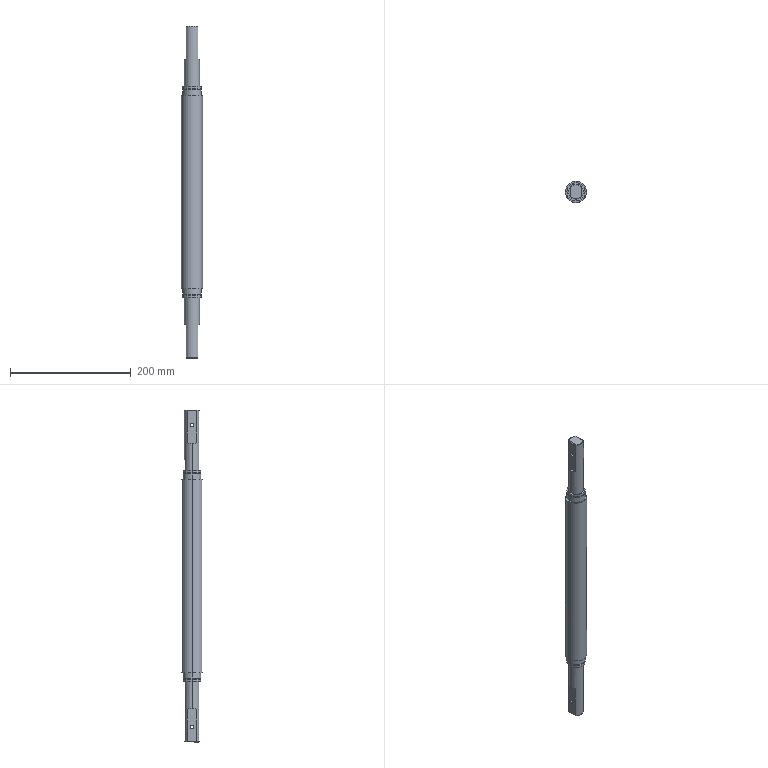Part | STEP file | Shaft 2 | 1 solid | 49 faces | box 35 x 35 x 550 mm | volume 418334 mm3 | cylinder 22 | plane 22 | cone 5 | commonest cylinder face diameters 30 x8 6 x4 25 x4 27.6 x4 35 x2
STEP:
#1=CARTESIAN_POINT('',(-17.5,0.,335.));
#2=VERTEX_POINT('',#1);
#3=CARTESIAN_POINT('',(17.5,0.,335.));
#4=VERTEX_POINT('',#3);
#5=CARTESIAN_POINT('',(0.,0.,335.));
#6=DIRECTION('',(0.,0.,-1.));
#7=DIRECTION('',(-1.,0.,0.));
#8=AXIS2_PLACEMENT_3D('',#5,#6,#7);
#9=CIRCLE('',#8,17.5);
#10=EDGE_CURVE('',#2,#4,#9,.T.);
#11=ORIENTED_EDGE('',*,*,#10,.T.);
#12=CARTESIAN_POINT('',(17.5,0.,15.));
#13=VERTEX_POINT('',#12);
#14=CARTESIAN_POINT('',(17.5,0.,350.));
#15=DIRECTION('',(0.,0.,-1.));
#16=VECTOR('',#15,1000.);
#17=LINE('',#14,#16);
#18=EDGE_CURVE('',#4,#13,#17,.T.);
#19=ORIENTED_EDGE('',*,*,#18,.T.);
#20=CARTESIAN_POINT('',(-17.5,0.,15.));
#21=VERTEX_POINT('',#20);
#22=CARTESIAN_POINT('',(0.,0.,15.));
#23=DIRECTION('',(0.,0.,1.));
#24=DIRECTION('',(-1.,0.,0.));
#25=AXIS2_PLACEMENT_3D('',#22,#23,#24);
#26=CIRCLE('',#25,17.5);
#27=EDGE_CURVE('',#13,#21,#26,.T.);
#28=ORIENTED_EDGE('',*,*,#27,.T.);
#29=CARTESIAN_POINT('',(-17.5,0.,350.));
#30=DIRECTION('',(0.,0.,-1.));
#31=VECTOR('',#30,1000.);
#32=LINE('',#29,#31);
#33=EDGE_CURVE('',#2,#21,#32,.T.);
#34=ORIENTED_EDGE('',*,*,#33,.F.);
#35=EDGE_LOOP('',(#11,#19,#28,#34));
#36=FACE_OUTER_BOUND('',#35,.T.);
#37=CARTESIAN_POINT('',(0.,0.,350.));
#38=DIRECTION('',(0.,0.,-1.));
#39=DIRECTION('',(-1.,0.,0.));
#40=AXIS2_PLACEMENT_3D('',#37,#38,#39);
#41=CYLINDRICAL_SURFACE('',#40,17.5);
#42=ADVANCED_FACE('',(#36),#41,.T.);
#43=CARTESIAN_POINT('',(15.,0.,15.));
#44=VERTEX_POINT('',#43);
#45=CARTESIAN_POINT('',(-15.,0.,15.));
#46=VERTEX_POINT('',#45);
#47=CARTESIAN_POINT('',(0.,0.,15.));
#48=DIRECTION('',(0.,0.,1.));
#49=DIRECTION('',(-1.,0.,0.));
#50=AXIS2_PLACEMENT_3D('',#47,#48,#49);
#51=CIRCLE('',#50,15.);
#52=EDGE_CURVE('',#44,#46,#51,.T.);
#53=ORIENTED_EDGE('',*,*,#52,.F.);
#54=CARTESIAN_POINT('',(15.,0.,6.));
#55=VERTEX_POINT('',#54);
#56=CARTESIAN_POINT('',(15.,0.,15.));
#57=DIRECTION('',(0.,0.,-1.));
#58=VECTOR('',#57,1000.);
#59=LINE('',#56,#58);
#60=EDGE_CURVE('',#44,#55,#59,.T.);
#61=ORIENTED_EDGE('',*,*,#60,.T.);
#62=CARTESIAN_POINT('',(-15.,0.,6.));
#63=VERTEX_POINT('',#62);
#64=CARTESIAN_POINT('',(0.,0.,6.));
#65=DIRECTION('',(0.,0.,1.));
#66=DIRECTION('',(-1.,0.,0.));
#67=AXIS2_PLACEMENT_3D('',#64,#65,#66);
#68=CIRCLE('',#67,15.);
#69=EDGE_CURVE('',#55,#63,#68,.T.);
#70=ORIENTED_EDGE('',*,*,#69,.T.);
#71=CARTESIAN_POINT('',(-15.,0.,15.));
#72=DIRECTION('',(0.,0.,-1.));
#73=VECTOR('',#72,1000.);
#74=LINE('',#71,#73);
#75=EDGE_CURVE('',#46,#63,#74,.T.);
#76=ORIENTED_EDGE('',*,*,#75,.F.);
#77=EDGE_LOOP('',(#53,#61,#70,#76));
#78=FACE_OUTER_BOUND('',#77,.T.);
#79=CARTESIAN_POINT('',(0.,0.,15.));
#80=DIRECTION('',(0.,0.,-1.));
#81=DIRECTION('',(-1.,0.,0.));
#82=AXIS2_PLACEMENT_3D('',#79,#80,#81);
#83=CYLINDRICAL_SURFACE('',#82,15.);
#84=ADVANCED_FACE('',(#78),#83,.T.);
#85=CARTESIAN_POINT('',(-15.,0.,335.));
#86=VERTEX_POINT('',#85);
#87=CARTESIAN_POINT('',(15.,0.,335.));
#88=VERTEX_POINT('',#87);
#89=CARTESIAN_POINT('',(0.,0.,335.));
#90=DIRECTION('',(0.,0.,-1.));
#91=DIRECTION('',(1.,0.,0.));
#92=AXIS2_PLACEMENT_3D('',#89,#90,#91);
#93=CIRCLE('',#92,15.);
#94=EDGE_CURVE('',#86,#88,#93,.T.);
#95=ORIENTED_EDGE('',*,*,#94,.F.);
#96=CARTESIAN_POINT('',(-15.,0.,344.));
#97=VERTEX_POINT('',#96);
#98=CARTESIAN_POINT('',(-15.,0.,335.));
#99=DIRECTION('',(0.,0.,1.));
#100=VECTOR('',#99,1000.);
#101=LINE('',#98,#100);
#102=EDGE_CURVE('',#86,#97,#101,.T.);
#103=ORIENTED_EDGE('',*,*,#102,.T.);
#104=CARTESIAN_POINT('',(15.,0.,344.));
#105=VERTEX_POINT('',#104);
#106=CARTESIAN_POINT('',(0.,0.,344.));
#107=DIRECTION('',(0.,0.,-1.));
#108=DIRECTION('',(1.,0.,0.));
#109=AXIS2_PLACEMENT_3D('',#106,#107,#108);
#110=CIRCLE('',#109,15.);
#111=EDGE_CURVE('',#97,#105,#110,.T.);
#112=ORIENTED_EDGE('',*,*,#111,.T.);
#113=CARTESIAN_POINT('',(15.,0.,335.));
#114=DIRECTION('',(0.,0.,1.));
#115=VECTOR('',#114,1000.);
#116=LINE('',#113,#115);
#117=EDGE_CURVE('',#88,#105,#116,.T.);
#118=ORIENTED_EDGE('',*,*,#117,.F.);
#119=EDGE_LOOP('',(#95,#103,#112,#118));
#120=FACE_OUTER_BOUND('',#119,.T.);
#121=CARTESIAN_POINT('',(0.,0.,335.));
#122=DIRECTION('',(0.,0.,1.));
#123=DIRECTION('',(1.,0.,0.));
#124=AXIS2_PLACEMENT_3D('',#121,#122,#123);
#125=CYLINDRICAL_SURFACE('',#124,15.);
#126=ADVANCED_FACE('',(#120),#125,.T.);
#127=CARTESIAN_POINT('',(-13.8,0.,6.));
#128=VERTEX_POINT('',#127);
#129=CARTESIAN_POINT('',(13.8,0.,6.));
#130=VERTEX_POINT('',#129);
#131=CARTESIAN_POINT('',(0.,0.,6.));
#132=DIRECTION('',(0.,0.,-1.));
#133=DIRECTION('',(-1.,0.,0.));
#134=AXIS2_PLACEMENT_3D('',#131,#132,#133);
#135=CIRCLE('',#134,13.8);
#136=EDGE_CURVE('',#128,#130,#135,.T.);
#137=ORIENTED_EDGE('',*,*,#136,.T.);
#138=CARTESIAN_POINT('',(13.8,0.,4.));
#139=VERTEX_POINT('',#138);
#140=CARTESIAN_POINT('',(13.8,0.,-86.604));
#141=DIRECTION('',(0.,0.,-1.));
#142=VECTOR('',#141,1000.);
#143=LINE('',#140,#142);
#144=EDGE_CURVE('',#130,#139,#143,.T.);
#145=ORIENTED_EDGE('',*,*,#144,.T.);
#146=CARTESIAN_POINT('',(-13.8,0.,4.));
#147=VERTEX_POINT('',#146);
#148=CARTESIAN_POINT('',(0.,0.,4.));
#149=DIRECTION('',(0.,0.,1.));
#150=DIRECTION('',(-1.,0.,0.));
#151=AXIS2_PLACEMENT_3D('',#148,#149,#150);
#152=CIRCLE('',#151,13.8);
#153=EDGE_CURVE('',#139,#147,#152,.T.);
#154=ORIENTED_EDGE('',*,*,#153,.T.);
#155=CARTESIAN_POINT('',(-13.8,0.,-86.604));
#156=DIRECTION('',(0.,0.,-1.));
#157=VECTOR('',#156,1000.);
#158=LINE('',#155,#157);
#159=EDGE_CURVE('',#128,#147,#158,.T.);
#160=ORIENTED_EDGE('',*,*,#159,.F.);
#161=EDGE_LOOP('',(#137,#145,#154,#160));
#162=FACE_OUTER_BOUND('',#161,.T.);
#163=CARTESIAN_POINT('',(0.,0.,-86.604));
#164=DIRECTION('',(0.,0.,-1.));
#165=DIRECTION('',(-1.,0.,0.));
#166=AXIS2_PLACEMENT_3D('',#163,#164,#165);
#167=CYLINDRICAL_SURFACE('',#166,13.8);
#168=ADVANCED_FACE('',(#162),#167,.T.);
#169=CARTESIAN_POINT('',(-13.8,0.,346.));
#170=VERTEX_POINT('',#169);
#171=CARTESIAN_POINT('',(13.8,0.,346.));
#172=VERTEX_POINT('',#171);
#173=CARTESIAN_POINT('',(0.,0.,346.));
#174=DIRECTION('',(0.,0.,-1.));
#175=DIRECTION('',(-1.,0.,0.));
#176=AXIS2_PLACEMENT_3D('',#173,#174,#175);
#177=CIRCLE('',#176,13.8);
#178=EDGE_CURVE('',#170,#172,#177,.T.);
#179=ORIENTED_EDGE('',*,*,#178,.T.);
#180=CARTESIAN_POINT('',(13.8,0.,344.));
#181=VERTEX_POINT('',#180);
#182=CARTESIAN_POINT('',(13.8,0.,-86.604));
#183=DIRECTION('',(0.,0.,-1.));
#184=VECTOR('',#183,1000.);
#185=LINE('',#182,#184);
#186=EDGE_CURVE('',#172,#181,#185,.T.);
#187=ORIENTED_EDGE('',*,*,#186,.T.);
#188=CARTESIAN_POINT('',(-13.8,0.,344.));
#189=VERTEX_POINT('',#188);
#190=CARTESIAN_POINT('',(0.,0.,344.));
#191=DIRECTION('',(0.,0.,1.));
#192=DIRECTION('',(-1.,0.,0.));
#193=AXIS2_PLACEMENT_3D('',#190,#191,#192);
#194=CIRCLE('',#193,13.8);
#195=EDGE_CURVE('',#181,#189,#194,.T.);
#196=ORIENTED_EDGE('',*,*,#195,.T.);
#197=CARTESIAN_POINT('',(-13.8,0.,-86.604));
#198=DIRECTION('',(0.,0.,-1.));
#199=VECTOR('',#198,1000.);
#200=LINE('',#197,#199);
#201=EDGE_CURVE('',#170,#189,#200,.T.);
#202=ORIENTED_EDGE('',*,*,#201,.F.);
#203=EDGE_LOOP('',(#179,#187,#196,#202));
#204=FACE_OUTER_BOUND('',#203,.T.);
#205=CARTESIAN_POINT('',(0.,0.,-86.604));
#206=DIRECTION('',(0.,0.,-1.));
#207=DIRECTION('',(-1.,0.,0.));
#208=AXIS2_PLACEMENT_3D('',#205,#206,#207);
#209=CYLINDRICAL_SURFACE('',#208,13.8);
#210=ADVANCED_FACE('',(#204),#209,.T.);
#211=CARTESIAN_POINT('',(-15.,0.,4.));
#212=VERTEX_POINT('',#211);
#213=CARTESIAN_POINT('',(15.,0.,4.));
#214=VERTEX_POINT('',#213);
#215=CARTESIAN_POINT('',(0.,0.,4.));
#216=DIRECTION('',(0.,0.,-1.));
#217=DIRECTION('',(-1.,0.,0.));
#218=AXIS2_PLACEMENT_3D('',#215,#216,#217);
#219=CIRCLE('',#218,15.);
#220=EDGE_CURVE('',#212,#214,#219,.T.);
#221=ORIENTED_EDGE('',*,*,#220,.T.);
#222=CARTESIAN_POINT('',(15.,0.,0.));
#223=VERTEX_POINT('',#222);
#224=CARTESIAN_POINT('',(15.,0.,15.));
#225=DIRECTION('',(0.,0.,-1.));
#226=VECTOR('',#225,1000.);
#227=LINE('',#224,#226);
#228=EDGE_CURVE('',#214,#223,#227,.T.);
#229=ORIENTED_EDGE('',*,*,#228,.T.);
#230=CARTESIAN_POINT('',(-15.,0.,0.));
#231=VERTEX_POINT('',#230);
#232=CARTESIAN_POINT('',(0.,0.,0.));
#233=DIRECTION('',(0.,0.,1.));
#234=DIRECTION('',(-1.,0.,0.));
#235=AXIS2_PLACEMENT_3D('',#232,#233,#234);
#236=CIRCLE('',#235,15.);
#237=EDGE_CURVE('',#223,#231,#236,.T.);
#238=ORIENTED_EDGE('',*,*,#237,.T.);
#239=CARTESIAN_POINT('',(-15.,0.,15.));
#240=DIRECTION('',(0.,0.,-1.));
#241=VECTOR('',#240,1000.);
#242=LINE('',#239,#241);
#243=EDGE_CURVE('',#212,#231,#242,.T.);
#244=ORIENTED_EDGE('',*,*,#243,.F.);
#245=EDGE_LOOP('',(#221,#229,#238,#244));
#246=FACE_OUTER_BOUND('',#245,.T.);
#247=CARTESIAN_POINT('',(0.,0.,15.));
#248=DIRECTION('',(0.,0.,-1.));
#249=DIRECTION('',(-1.,0.,0.));
#250=AXIS2_PLACEMENT_3D('',#247,#248,#249);
#251=CYLINDRICAL_SURFACE('',#250,15.);
#252=ADVANCED_FACE('',(#246),#251,.T.);
#253=CARTESIAN_POINT('',(15.,0.,346.));
#254=VERTEX_POINT('',#253);
#255=CARTESIAN_POINT('',(-15.,0.,346.));
#256=VERTEX_POINT('',#255);
#257=CARTESIAN_POINT('',(0.,0.,346.));
#258=DIRECTION('',(0.,0.,1.));
#259=DIRECTION('',(1.,0.,0.));
#260=AXIS2_PLACEMENT_3D('',#257,#258,#259);
#261=CIRCLE('',#260,15.);
#262=EDGE_CURVE('',#254,#256,#261,.T.);
#263=ORIENTED_EDGE('',*,*,#262,.T.);
#264=CARTESIAN_POINT('',(-15.,0.,350.));
#265=VERTEX_POINT('',#264);
#266=CARTESIAN_POINT('',(-15.,0.,335.));
#267=DIRECTION('',(0.,0.,1.));
#268=VECTOR('',#267,1000.);
#269=LINE('',#266,#268);
#270=EDGE_CURVE('',#256,#265,#269,.T.);
#271=ORIENTED_EDGE('',*,*,#270,.T.);
#272=CARTESIAN_POINT('',(15.,0.,350.));
#273=VERTEX_POINT('',#272);
#274=CARTESIAN_POINT('',(0.,0.,350.));
#275=DIRECTION('',(0.,0.,-1.));
#276=DIRECTION('',(1.,0.,0.));
#277=AXIS2_PLACEMENT_3D('',#274,#275,#276);
#278=CIRCLE('',#277,15.);
#279=EDGE_CURVE('',#265,#273,#278,.T.);
#280=ORIENTED_EDGE('',*,*,#279,.T.);
#281=CARTESIAN_POINT('',(15.,0.,335.));
#282=DIRECTION('',(0.,0.,1.));
#283=VECTOR('',#282,1000.);
#284=LINE('',#281,#283);
#285=EDGE_CURVE('',#254,#273,#284,.T.);
#286=ORIENTED_EDGE('',*,*,#285,.F.);
#287=EDGE_LOOP('',(#263,#271,#280,#286));
#288=FACE_OUTER_BOUND('',#287,.T.);
#289=CARTESIAN_POINT('',(0.,0.,335.));
#290=DIRECTION('',(0.,0.,1.));
#291=DIRECTION('',(1.,0.,0.));
#292=AXIS2_PLACEMENT_3D('',#289,#290,#291);
#293=CYLINDRICAL_SURFACE('',#292,15.);
#294=ADVANCED_FACE('',(#288),#293,.T.);
#295=CARTESIAN_POINT('',(-9.5,8.124,-45.));
#296=VERTEX_POINT('',#295);
#297=CARTESIAN_POINT('',(-12.5,0.,-45.));
#298=VERTEX_POINT('',#297);
#299=CARTESIAN_POINT('',(0.,0.,-45.));
#300=DIRECTION('',(0.,0.,1.));
#301=DIRECTION('',(1.,0.,0.));
#302=AXIS2_PLACEMENT_3D('',#299,#300,#301);
#303=CIRCLE('',#302,12.5);
#304=EDGE_CURVE('',#296,#298,#303,.T.);
#305=ORIENTED_EDGE('',*,*,#304,.T.);
#306=CARTESIAN_POINT('',(-12.5,0.,0.));
#307=VERTEX_POINT('',#306);
#308=CARTESIAN_POINT('',(-12.5,0.,-100.));
#309=DIRECTION('',(0.,0.,1.));
#310=VECTOR('',#309,1000.);
#311=LINE('',#308,#310);
#312=EDGE_CURVE('',#298,#307,#311,.T.);
#313=ORIENTED_EDGE('',*,*,#312,.T.);
#314=CARTESIAN_POINT('',(12.5,0.,0.));
#315=VERTEX_POINT('',#314);
#316=CARTESIAN_POINT('',(0.,0.,0.));
#317=DIRECTION('',(0.,0.,-1.));
#318=DIRECTION('',(1.,0.,0.));
#319=AXIS2_PLACEMENT_3D('',#316,#317,#318);
#320=CIRCLE('',#319,12.5);
#321=EDGE_CURVE('',#307,#315,#320,.T.);
#322=ORIENTED_EDGE('',*,*,#321,.T.);
#323=CARTESIAN_POINT('',(12.5,0.,-45.));
#324=VERTEX_POINT('',#323);
#325=CARTESIAN_POINT('',(12.5,0.,-100.));
#326=DIRECTION('',(0.,0.,1.));
#327=VECTOR('',#326,1000.);
#328=LINE('',#325,#327);
#329=EDGE_CURVE('',#324,#315,#328,.T.);
#330=ORIENTED_EDGE('',*,*,#329,.F.);
#331=CARTESIAN_POINT('',(9.5,8.124,-45.));
#332=VERTEX_POINT('',#331);
#333=CARTESIAN_POINT('',(0.,0.,-45.));
#334=DIRECTION('',(0.,0.,1.));
#335=DIRECTION('',(1.,0.,0.));
#336=AXIS2_PLACEMENT_3D('',#333,#334,#335);
#337=CIRCLE('',#336,12.5);
#338=EDGE_CURVE('',#324,#332,#337,.T.);
#339=ORIENTED_EDGE('',*,*,#338,.T.);
#340=CARTESIAN_POINT('',(9.5,8.124,-99.));
#341=VERTEX_POINT('',#340);
#342=CARTESIAN_POINT('',(9.5,8.124,-100.));
#343=DIRECTION('',(0.,0.,-1.));
#344=VECTOR('',#343,1000.);
#345=LINE('',#342,#344);
#346=EDGE_CURVE('',#332,#341,#345,.T.);
#347=ORIENTED_EDGE('',*,*,#346,.T.);
#348=CARTESIAN_POINT('',(-9.5,8.124,-99.));
#349=VERTEX_POINT('',#348);
#350=CARTESIAN_POINT('',(0.,0.,-99.));
#351=DIRECTION('',(0.,0.,1.));
#352=DIRECTION('',(1.,0.,0.));
#353=AXIS2_PLACEMENT_3D('',#350,#351,#352);
#354=CIRCLE('',#353,12.5);
#355=EDGE_CURVE('',#341,#349,#354,.T.);
#356=ORIENTED_EDGE('',*,*,#355,.T.);
#357=CARTESIAN_POINT('',(-9.5,8.124,-100.));
#358=DIRECTION('',(0.,0.,1.));
#359=VECTOR('',#358,1000.);
#360=LINE('',#357,#359);
#361=EDGE_CURVE('',#349,#296,#360,.T.);
#362=ORIENTED_EDGE('',*,*,#361,.T.);
#363=EDGE_LOOP('',(#305,#313,#322,#330,#339,#347,#356,#362));
#364=FACE_OUTER_BOUND('',#363,.T.);
#365=CARTESIAN_POINT('',(0.,0.,-100.));
#366=DIRECTION('',(0.,0.,1.));
#367=DIRECTION('',(1.,0.,0.));
#368=AXIS2_PLACEMENT_3D('',#365,#366,#367);
#369=CYLINDRICAL_SURFACE('',#368,12.5);
#370=ADVANCED_FACE('',(#364),#369,.T.);
#371=CARTESIAN_POINT('',(9.5,8.124,395.));
#372=VERTEX_POINT('',#371);
#373=CARTESIAN_POINT('',(12.5,0.,395.));
#374=VERTEX_POINT('',#373);
#375=CARTESIAN_POINT('',(0.,0.,395.));
#376=DIRECTION('',(0.,0.,-1.));
#377=DIRECTION('',(-1.,0.,0.));
#378=AXIS2_PLACEMENT_3D('',#375,#376,#377);
#379=CIRCLE('',#378,12.5);
#380=EDGE_CURVE('',#372,#374,#379,.T.);
#381=ORIENTED_EDGE('',*,*,#380,.T.);
#382=CARTESIAN_POINT('',(12.5,0.,350.));
#383=VERTEX_POINT('',#382);
#384=CARTESIAN_POINT('',(12.5,0.,450.));
#385=DIRECTION('',(0.,0.,-1.));
#386=VECTOR('',#385,1000.);
#387=LINE('',#384,#386);
#388=EDGE_CURVE('',#374,#383,#387,.T.);
#389=ORIENTED_EDGE('',*,*,#388,.T.);
#390=CARTESIAN_POINT('',(-12.5,0.,350.));
#391=VERTEX_POINT('',#390);
#392=CARTESIAN_POINT('',(0.,0.,350.));
#393=DIRECTION('',(0.,0.,-1.));
#394=DIRECTION('',(-1.,0.,0.));
#395=AXIS2_PLACEMENT_3D('',#392,#393,#394);
#396=CIRCLE('',#395,12.5);
#397=EDGE_CURVE('',#391,#383,#396,.T.);
#398=ORIENTED_EDGE('',*,*,#397,.F.);
#399=CARTESIAN_POINT('',(-12.5,0.,395.));
#400=VERTEX_POINT('',#399);
#401=CARTESIAN_POINT('',(-12.5,0.,450.));
#402=DIRECTION('',(0.,0.,-1.));
#403=VECTOR('',#402,1000.);
#404=LINE('',#401,#403);
#405=EDGE_CURVE('',#400,#391,#404,.T.);
#406=ORIENTED_EDGE('',*,*,#405,.F.);
#407=CARTESIAN_POINT('',(-9.5,8.124,395.));
#408=VERTEX_POINT('',#407);
#409=CARTESIAN_POINT('',(0.,0.,395.));
#410=DIRECTION('',(0.,0.,-1.));
#411=DIRECTION('',(-1.,0.,0.));
#412=AXIS2_PLACEMENT_3D('',#409,#410,#411);
#413=CIRCLE('',#412,12.5);
#414=EDGE_CURVE('',#400,#408,#413,.T.);
#415=ORIENTED_EDGE('',*,*,#414,.T.);
#416=CARTESIAN_POINT('',(-9.5,8.124,449.));
#417=VERTEX_POINT('',#416);
#418=CARTESIAN_POINT('',(-9.5,8.124,450.));
#419=DIRECTION('',(0.,0.,1.));
#420=VECTOR('',#419,1000.);
#421=LINE('',#418,#420);
#422=EDGE_CURVE('',#408,#417,#421,.T.);
#423=ORIENTED_EDGE('',*,*,#422,.T.);
#424=CARTESIAN_POINT('',(0.,12.5,449.));
#425=VERTEX_POINT('',#424);
#426=CARTESIAN_POINT('',(0.,0.,449.));
#427=DIRECTION('',(0.,0.,-1.));
#428=DIRECTION('',(-1.,0.,0.));
#429=AXIS2_PLACEMENT_3D('',#426,#427,#428);
#430=CIRCLE('',#429,12.5);
#431=EDGE_CURVE('',#417,#425,#430,.T.);
#432=ORIENTED_EDGE('',*,*,#431,.T.);
#433=CARTESIAN_POINT('',(9.5,8.124,449.));
#434=VERTEX_POINT('',#433);
#435=CARTESIAN_POINT('',(0.,0.,449.));
#436=DIRECTION('',(0.,0.,-1.));
#437=DIRECTION('',(-1.,0.,0.));
#438=AXIS2_PLACEMENT_3D('',#435,#436,#437);
#439=CIRCLE('',#438,12.5);
#440=EDGE_CURVE('',#425,#434,#439,.T.);
#441=ORIENTED_EDGE('',*,*,#440,.T.);
#442=CARTESIAN_POINT('',(9.5,8.124,450.));
#443=DIRECTION('',(0.,0.,-1.));
#444=VECTOR('',#443,1000.);
#445=LINE('',#442,#444);
#446=EDGE_CURVE('',#434,#372,#445,.T.);
#447=ORIENTED_EDGE('',*,*,#446,.T.);
#448=EDGE_LOOP('',(#381,#389,#398,#406,#415,#423,#432,#441,#447));
#449=FACE_OUTER_BOUND('',#448,.T.);
#450=CARTESIAN_POINT('',(0.,0.,450.));
#451=DIRECTION('',(0.,0.,-1.));
#452=DIRECTION('',(-1.,0.,0.));
#453=AXIS2_PLACEMENT_3D('',#450,#451,#452);
#454=CYLINDRICAL_SURFACE('',#453,12.5);
#455=ADVANCED_FACE('',(#449),#454,.T.);
#456=CARTESIAN_POINT('',(-8.5,7.746,450.));
#457=VERTEX_POINT('',#456);
#458=CARTESIAN_POINT('',(0.,11.5,450.));
#459=VERTEX_POINT('',#458);
#460=CARTESIAN_POINT('',(0.,0.,450.));
#461=DIRECTION('',(0.,0.,-1.));
#462=DIRECTION('',(0.,1.,0.));
#463=AXIS2_PLACEMENT_3D('',#460,#461,#462);
#464=CIRCLE('',#463,11.5);
#465=EDGE_CURVE('',#457,#459,#464,.T.);
#466=ORIENTED_EDGE('',*,*,#465,.T.);
#467=CARTESIAN_POINT('',(0.,12.5,449.));
#468=DIRECTION('',(0.,0.7071,-0.7071));
#469=VECTOR('',#468,1000.);
#470=LINE('',#467,#469);
#471=EDGE_CURVE('',#459,#425,#470,.T.);
#472=ORIENTED_EDGE('',*,*,#471,.T.);
#473=ORIENTED_EDGE('',*,*,#431,.F.);
#474=CARTESIAN_POINT('',(-8.5,7.746,450.));
#475=CARTESIAN_POINT('',(-8.833,7.875,449.667));
#476=CARTESIAN_POINT('',(-9.166,8.001,449.334));
#477=CARTESIAN_POINT('',(-9.5,8.124,449.));
#478=B_SPLINE_CURVE_WITH_KNOTS('',3,(#474,#475,#476,#477),.UNSPECIFIED.,.F.,.F.,(4,4),(0.,0.001464),.UNSPECIFIED.);
#479=EDGE_CURVE('',#457,#417,#478,.T.);
#480=ORIENTED_EDGE('',*,*,#479,.F.);
#481=EDGE_LOOP('',(#466,#472,#473,#480));
#482=FACE_OUTER_BOUND('',#481,.T.);
#483=CARTESIAN_POINT('',(0.,0.,449.));
#484=DIRECTION('',(0.,0.,-1.));
#485=DIRECTION('',(0.,1.,0.));
#486=AXIS2_PLACEMENT_3D('',#483,#484,#485);
#487=CONICAL_SURFACE('',#486,12.5,0.7854);
#488=ADVANCED_FACE('',(#482),#487,.T.);
#489=CARTESIAN_POINT('',(-9.5,0.,-78.));
#490=VERTEX_POINT('',#489);
#491=CARTESIAN_POINT('',(-9.5,0.,-72.));
#492=VERTEX_POINT('',#491);
#493=CARTESIAN_POINT('',(-9.5,0.,-75.));
#494=DIRECTION('',(-1.,0.,0.));
#495=DIRECTION('',(0.,0.,-1.));
#496=AXIS2_PLACEMENT_3D('',#493,#494,#495);
#497=CIRCLE('',#496,3.);
#498=EDGE_CURVE('',#490,#492,#497,.T.);
#499=ORIENTED_EDGE('',*,*,#498,.T.);
#500=CARTESIAN_POINT('',(9.5,0.,-72.));
#501=VERTEX_POINT('',#500);
#502=CARTESIAN_POINT('',(-10.5,0.,-72.));
#503=DIRECTION('',(1.,0.,0.));
#504=VECTOR('',#503,1000.);
#505=LINE('',#502,#504);
#506=EDGE_CURVE('',#492,#501,#505,.T.);
#507=ORIENTED_EDGE('',*,*,#506,.T.);
#508=CARTESIAN_POINT('',(9.5,0.,-78.));
#509=VERTEX_POINT('',#508);
#510=CARTESIAN_POINT('',(9.5,0.,-75.));
#511=DIRECTION('',(1.,0.,0.));
#512=DIRECTION('',(0.,0.,-1.));
#513=AXIS2_PLACEMENT_3D('',#510,#511,#512);
#514=CIRCLE('',#513,3.);
#515=EDGE_CURVE('',#501,#509,#514,.T.);
#516=ORIENTED_EDGE('',*,*,#515,.T.);
#517=CARTESIAN_POINT('',(-10.5,0.,-78.));
#518=DIRECTION('',(1.,0.,0.));
#519=VECTOR('',#518,1000.);
#520=LINE('',#517,#519);
#521=EDGE_CURVE('',#490,#509,#520,.T.);
#522=ORIENTED_EDGE('',*,*,#521,.F.);
#523=EDGE_LOOP('',(#499,#507,#516,#522));
#524=FACE_OUTER_BOUND('',#523,.T.);
#525=CARTESIAN_POINT('',(-10.5,0.,-75.));
#526=DIRECTION('',(1.,0.,0.));
#527=DIRECTION('',(0.,0.,-1.));
#528=AXIS2_PLACEMENT_3D('',#525,#526,#527);
#529=CYLINDRICAL_SURFACE('',#528,3.);
#530=ADVANCED_FACE('',(#524),#529,.F.);
#531=CARTESIAN_POINT('',(-9.5,0.,422.));
#532=VERTEX_POINT('',#531);
#533=CARTESIAN_POINT('',(-9.5,0.,428.));
#534=VERTEX_POINT('',#533);
#535=CARTESIAN_POINT('',(-9.5,0.,425.));
#536=DIRECTION('',(-1.,0.,0.));
#537=DIRECTION('',(0.,0.,-1.));
#538=AXIS2_PLACEMENT_3D('',#535,#536,#537);
#539=CIRCLE('',#538,3.);
#540=EDGE_CURVE('',#532,#534,#539,.T.);
#541=ORIENTED_EDGE('',*,*,#540,.T.);
#542=CARTESIAN_POINT('',(9.5,0.,428.));
#543=VERTEX_POINT('',#542);
#544=CARTESIAN_POINT('',(-10.5,0.,428.));
#545=DIRECTION('',(1.,0.,0.));
#546=VECTOR('',#545,1000.);
#547=LINE('',#544,#546);
#548=EDGE_CURVE('',#534,#543,#547,.T.);
#549=ORIENTED_EDGE('',*,*,#548,.T.);
#550=CARTESIAN_POINT('',(9.5,0.,422.));
#551=VERTEX_POINT('',#550);
#552=CARTESIAN_POINT('',(9.5,0.,425.));
#553=DIRECTION('',(1.,0.,0.));
#554=DIRECTION('',(0.,0.,-1.));
#555=AXIS2_PLACEMENT_3D('',#552,#553,#554);
#556=CIRCLE('',#555,3.);
#557=EDGE_CURVE('',#543,#551,#556,.T.);
#558=ORIENTED_EDGE('',*,*,#557,.T.);
#559=CARTESIAN_POINT('',(-10.5,0.,422.));
#560=DIRECTION('',(1.,0.,0.));
#561=VECTOR('',#560,1000.);
#562=LINE('',#559,#561);
#563=EDGE_CURVE('',#532,#551,#562,.T.);
#564=ORIENTED_EDGE('',*,*,#563,.F.);
#565=EDGE_LOOP('',(#541,#549,#558,#564));
#566=FACE_OUTER_BOUND('',#565,.T.);
#567=CARTESIAN_POINT('',(-10.5,0.,425.));
#568=DIRECTION('',(1.,0.,0.));
#569=DIRECTION('',(0.,0.,-1.));
#570=AXIS2_PLACEMENT_3D('',#567,#568,#569);
#571=CYLINDRICAL_SURFACE('',#570,3.);
#572=ADVANCED_FACE('',(#566),#571,.F.);
#573=ORIENTED_EDGE('',*,*,#18,.F.);
#574=CARTESIAN_POINT('',(0.,0.,335.));
#575=DIRECTION('',(0.,0.,-1.));
#576=DIRECTION('',(-1.,0.,0.));
#577=AXIS2_PLACEMENT_3D('',#574,#575,#576);
#578=CIRCLE('',#577,17.5);
#579=EDGE_CURVE('',#4,#2,#578,.T.);
#580=ORIENTED_EDGE('',*,*,#579,.T.);
#581=ORIENTED_EDGE('',*,*,#33,.T.);
#582=CARTESIAN_POINT('',(0.,0.,15.));
#583=DIRECTION('',(0.,0.,1.));
#584=DIRECTION('',(-1.,0.,0.));
#585=AXIS2_PLACEMENT_3D('',#582,#583,#584);
#586=CIRCLE('',#585,17.5);
#587=EDGE_CURVE('',#21,#13,#586,.T.);
#588=ORIENTED_EDGE('',*,*,#587,.T.);
#589=EDGE_LOOP('',(#573,#580,#581,#588));
#590=FACE_OUTER_BOUND('',#589,.T.);
#591=CARTESIAN_POINT('',(0.,0.,350.));
#592=DIRECTION('',(0.,0.,-1.));
#593=DIRECTION('',(-1.,0.,0.));
#594=AXIS2_PLACEMENT_3D('',#591,#592,#593);
#595=CYLINDRICAL_SURFACE('',#594,17.5);
#596=ADVANCED_FACE('',(#590),#595,.T.);
#597=ORIENTED_EDGE('',*,*,#587,.F.);
#598=ORIENTED_EDGE('',*,*,#27,.F.);
#599=EDGE_LOOP('',(#597,#598));
#600=FACE_OUTER_BOUND('',#599,.T.);
#601=CARTESIAN_POINT('',(0.,0.,15.));
#602=DIRECTION('',(0.,0.,1.));
#603=DIRECTION('',(-1.,0.,0.));
#604=AXIS2_PLACEMENT_3D('',#601,#602,#603);
#605=CIRCLE('',#604,15.);
#606=EDGE_CURVE('',#46,#44,#605,.T.);
#607=ORIENTED_EDGE('',*,*,#606,.T.);
#608=ORIENTED_EDGE('',*,*,#52,.T.);
#609=EDGE_LOOP('',(#607,#608));
#610=FACE_BOUND('',#609,.T.);
#611=CARTESIAN_POINT('',(0.,0.,15.));
#612=DIRECTION('',(0.,0.,-1.));
#613=DIRECTION('',(-1.,0.,0.));
#614=AXIS2_PLACEMENT_3D('',#611,#612,#613);
#615=PLANE('',#614);
#616=ADVANCED_FACE('',(#600,#610),#615,.T.);
#617=ORIENTED_EDGE('',*,*,#10,.F.);
#618=ORIENTED_EDGE('',*,*,#579,.F.);
#619=EDGE_LOOP('',(#617,#618));
#620=FACE_OUTER_BOUND('',#619,.T.);
#621=CARTESIAN_POINT('',(0.,0.,335.));
#622=DIRECTION('',(0.,0.,-1.));
#623=DIRECTION('',(1.,0.,0.));
#624=AXIS2_PLACEMENT_3D('',#621,#622,#623);
#625=CIRCLE('',#624,15.);
#626=EDGE_CURVE('',#88,#86,#625,.T.);
#627=ORIENTED_EDGE('',*,*,#626,.T.);
#628=ORIENTED_EDGE('',*,*,#94,.T.);
#629=EDGE_LOOP('',(#627,#628));
#630=FACE_BOUND('',#629,.T.);
#631=CARTESIAN_POINT('',(0.,0.,335.));
#632=DIRECTION('',(0.,0.,1.));
#633=DIRECTION('',(1.,0.,0.));
#634=AXIS2_PLACEMENT_3D('',#631,#632,#633);
#635=PLANE('',#634);
#636=ADVANCED_FACE('',(#620,#630),#635,.T.);
#637=ORIENTED_EDGE('',*,*,#60,.F.);
#638=ORIENTED_EDGE('',*,*,#606,.F.);
#639=ORIENTED_EDGE('',*,*,#75,.T.);
#640=CARTESIAN_POINT('',(0.,0.,6.));
#641=DIRECTION('',(0.,0.,1.));
#642=DIRECTION('',(-1.,0.,0.));
#643=AXIS2_PLACEMENT_3D('',#640,#641,#642);
#644=CIRCLE('',#643,15.);
#645=EDGE_CURVE('',#63,#55,#644,.T.);
#646=ORIENTED_EDGE('',*,*,#645,.T.);
#647=EDGE_LOOP('',(#637,#638,#639,#646));
#648=FACE_OUTER_BOUND('',#647,.T.);
#649=CARTESIAN_POINT('',(0.,0.,15.));
#650=DIRECTION('',(0.,0.,-1.));
#651=DIRECTION('',(-1.,0.,0.));
#652=AXIS2_PLACEMENT_3D('',#649,#650,#651);
#653=CYLINDRICAL_SURFACE('',#652,15.);
#654=ADVANCED_FACE('',(#648),#653,.T.);
#655=ORIENTED_EDGE('',*,*,#102,.F.);
#656=ORIENTED_EDGE('',*,*,#626,.F.);
#657=ORIENTED_EDGE('',*,*,#117,.T.);
#658=CARTESIAN_POINT('',(0.,0.,344.));
#659=DIRECTION('',(0.,0.,-1.));
#660=DIRECTION('',(1.,0.,0.));
#661=AXIS2_PLACEMENT_3D('',#658,#659,#660);
#662=CIRCLE('',#661,15.);
#663=EDGE_CURVE('',#105,#97,#662,.T.);
#664=ORIENTED_EDGE('',*,*,#663,.T.);
#665=EDGE_LOOP('',(#655,#656,#657,#664));
#666=FACE_OUTER_BOUND('',#665,.T.);
#667=CARTESIAN_POINT('',(0.,0.,335.));
#668=DIRECTION('',(0.,0.,1.));
#669=DIRECTION('',(1.,0.,0.));
#670=AXIS2_PLACEMENT_3D('',#667,#668,#669);
#671=CYLINDRICAL_SURFACE('',#670,15.);
#672=ADVANCED_FACE('',(#666),#671,.T.);
#673=ORIENTED_EDGE('',*,*,#136,.F.);
#674=CARTESIAN_POINT('',(0.,0.,6.));
#675=DIRECTION('',(0.,0.,-1.));
#676=DIRECTION('',(-1.,0.,0.));
#677=AXIS2_PLACEMENT_3D('',#674,#675,#676);
#678=CIRCLE('',#677,13.8);
#679=EDGE_CURVE('',#130,#128,#678,.T.);
#680=ORIENTED_EDGE('',*,*,#679,.F.);
#681=EDGE_LOOP('',(#673,#680));
#682=FACE_BOUND('',#681,.T.);
#683=ORIENTED_EDGE('',*,*,#645,.F.);
#684=ORIENTED_EDGE('',*,*,#69,.F.);
#685=EDGE_LOOP('',(#683,#684));
#686=FACE_OUTER_BOUND('',#685,.T.);
#687=CARTESIAN_POINT('',(-15.3,0.,6.));
#688=DIRECTION('',(0.,0.,1.));
#689=DIRECTION('',(1.,0.,0.));
#690=AXIS2_PLACEMENT_3D('',#687,#688,#689);
#691=PLANE('',#690);
#692=ADVANCED_FACE('',(#682,#686),#691,.F.);
#693=CARTESIAN_POINT('',(0.,0.,344.));
#694=DIRECTION('',(0.,0.,1.));
#695=DIRECTION('',(-1.,0.,0.));
#696=AXIS2_PLACEMENT_3D('',#693,#694,#695);
#697=CIRCLE('',#696,13.8);
#698=EDGE_CURVE('',#189,#181,#697,.T.);
#699=ORIENTED_EDGE('',*,*,#698,.F.);
#700=ORIENTED_EDGE('',*,*,#195,.F.);
#701=EDGE_LOOP('',(#699,#700));
#702=FACE_BOUND('',#701,.T.);
#703=ORIENTED_EDGE('',*,*,#663,.F.);
#704=ORIENTED_EDGE('',*,*,#111,.F.);
#705=EDGE_LOOP('',(#703,#704));
#706=FACE_OUTER_BOUND('',#705,.T.);
#707=CARTESIAN_POINT('',(-15.3,0.,344.));
#708=DIRECTION('',(0.,0.,-1.));
#709=DIRECTION('',(-1.,0.,0.));
#710=AXIS2_PLACEMENT_3D('',#707,#708,#709);
#711=PLANE('',#710);
#712=ADVANCED_FACE('',(#702,#706),#711,.F.);
#713=ORIENTED_EDGE('',*,*,#144,.F.);
#714=ORIENTED_EDGE('',*,*,#679,.T.);
#715=ORIENTED_EDGE('',*,*,#159,.T.);
#716=CARTESIAN_POINT('',(0.,0.,4.));
#717=DIRECTION('',(0.,0.,1.));
#718=DIRECTION('',(-1.,0.,0.));
#719=AXIS2_PLACEMENT_3D('',#716,#717,#718);
#720=CIRCLE('',#719,13.8);
#721=EDGE_CURVE('',#147,#139,#720,.T.);
#722=ORIENTED_EDGE('',*,*,#721,.T.);
#723=EDGE_LOOP('',(#713,#714,#715,#722));
#724=FACE_OUTER_BOUND('',#723,.T.);
#725=CARTESIAN_POINT('',(0.,0.,-86.604));
#726=DIRECTION('',(0.,0.,-1.));
#727=DIRECTION('',(-1.,0.,0.));
#728=AXIS2_PLACEMENT_3D('',#725,#726,#727);
#729=CYLINDRICAL_SURFACE('',#728,13.8);
#730=ADVANCED_FACE('',(#724),#729,.T.);
#731=ORIENTED_EDGE('',*,*,#186,.F.);
#732=CARTESIAN_POINT('',(0.,0.,346.));
#733=DIRECTION('',(0.,0.,-1.));
#734=DIRECTION('',(-1.,0.,0.));
#735=AXIS2_PLACEMENT_3D('',#732,#733,#734);
#736=CIRCLE('',#735,13.8);
#737=EDGE_CURVE('',#172,#170,#736,.T.);
#738=ORIENTED_EDGE('',*,*,#737,.T.);
#739=ORIENTED_EDGE('',*,*,#201,.T.);
#740=ORIENTED_EDGE('',*,*,#698,.T.);
#741=EDGE_LOOP('',(#731,#738,#739,#740));
#742=FACE_OUTER_BOUND('',#741,.T.);
#743=CARTESIAN_POINT('',(0.,0.,-86.604));
#744=DIRECTION('',(0.,0.,-1.));
#745=DIRECTION('',(-1.,0.,0.));
#746=AXIS2_PLACEMENT_3D('',#743,#744,#745);
#747=CYLINDRICAL_SURFACE('',#746,13.8);
#748=ADVANCED_FACE('',(#742),#747,.T.);
#749=ORIENTED_EDGE('',*,*,#721,.F.);
#750=ORIENTED_EDGE('',*,*,#153,.F.);
#751=EDGE_LOOP('',(#749,#750));
#752=FACE_BOUND('',#751,.T.);
#753=ORIENTED_EDGE('',*,*,#220,.F.);
#754=CARTESIAN_POINT('',(0.,0.,4.));
#755=DIRECTION('',(0.,0.,-1.));
#756=DIRECTION('',(-1.,0.,0.));
#757=AXIS2_PLACEMENT_3D('',#754,#755,#756);
#758=CIRCLE('',#757,15.);
#759=EDGE_CURVE('',#214,#212,#758,.T.);
#760=ORIENTED_EDGE('',*,*,#759,.F.);
#761=EDGE_LOOP('',(#753,#760));
#762=FACE_OUTER_BOUND('',#761,.T.);
#763=CARTESIAN_POINT('',(-15.3,0.,4.));
#764=DIRECTION('',(0.,0.,-1.));
#765=DIRECTION('',(-1.,0.,0.));
#766=AXIS2_PLACEMENT_3D('',#763,#764,#765);
#767=PLANE('',#766);
#768=ADVANCED_FACE('',(#752,#762),#767,.F.);
#769=ORIENTED_EDGE('',*,*,#178,.F.);
#770=ORIENTED_EDGE('',*,*,#737,.F.);
#771=EDGE_LOOP('',(#769,#770));
#772=FACE_BOUND('',#771,.T.);
#773=ORIENTED_EDGE('',*,*,#262,.F.);
#774=CARTESIAN_POINT('',(0.,0.,346.));
#775=DIRECTION('',(0.,0.,1.));
#776=DIRECTION('',(1.,0.,0.));
#777=AXIS2_PLACEMENT_3D('',#774,#775,#776);
#778=CIRCLE('',#777,15.);
#779=EDGE_CURVE('',#256,#254,#778,.T.);
#780=ORIENTED_EDGE('',*,*,#779,.F.);
#781=EDGE_LOOP('',(#773,#780));
#782=FACE_OUTER_BOUND('',#781,.T.);
#783=CARTESIAN_POINT('',(-15.3,0.,346.));
#784=DIRECTION('',(0.,0.,1.));
#785=DIRECTION('',(1.,0.,0.));
#786=AXIS2_PLACEMENT_3D('',#783,#784,#785);
#787=PLANE('',#786);
#788=ADVANCED_FACE('',(#772,#782),#787,.F.);
#789=ORIENTED_EDGE('',*,*,#228,.F.);
#790=ORIENTED_EDGE('',*,*,#759,.T.);
#791=ORIENTED_EDGE('',*,*,#243,.T.);
#792=CARTESIAN_POINT('',(0.,0.,0.));
#793=DIRECTION('',(0.,0.,1.));
#794=DIRECTION('',(-1.,0.,0.));
#795=AXIS2_PLACEMENT_3D('',#792,#793,#794);
#796=CIRCLE('',#795,15.);
#797=EDGE_CURVE('',#231,#223,#796,.T.);
#798=ORIENTED_EDGE('',*,*,#797,.T.);
#799=EDGE_LOOP('',(#789,#790,#791,#798));
#800=FACE_OUTER_BOUND('',#799,.T.);
#801=CARTESIAN_POINT('',(0.,0.,15.));
#802=DIRECTION('',(0.,0.,-1.));
#803=DIRECTION('',(-1.,0.,0.));
#804=AXIS2_PLACEMENT_3D('',#801,#802,#803);
#805=CYLINDRICAL_SURFACE('',#804,15.);
#806=ADVANCED_FACE('',(#800),#805,.T.);
#807=ORIENTED_EDGE('',*,*,#270,.F.);
#808=ORIENTED_EDGE('',*,*,#779,.T.);
#809=ORIENTED_EDGE('',*,*,#285,.T.);
#810=CARTESIAN_POINT('',(0.,0.,350.));
#811=DIRECTION('',(0.,0.,-1.));
#812=DIRECTION('',(1.,0.,0.));
#813=AXIS2_PLACEMENT_3D('',#810,#811,#812);
#814=CIRCLE('',#813,15.);
#815=EDGE_CURVE('',#273,#265,#814,.T.);
#816=ORIENTED_EDGE('',*,*,#815,.T.);
#817=EDGE_LOOP('',(#807,#808,#809,#816));
#818=FACE_OUTER_BOUND('',#817,.T.);
#819=CARTESIAN_POINT('',(0.,0.,335.));
#820=DIRECTION('',(0.,0.,1.));
#821=DIRECTION('',(1.,0.,0.));
#822=AXIS2_PLACEMENT_3D('',#819,#820,#821);
#823=CYLINDRICAL_SURFACE('',#822,15.);
#824=ADVANCED_FACE('',(#818),#823,.T.);
#825=ORIENTED_EDGE('',*,*,#797,.F.);
#826=ORIENTED_EDGE('',*,*,#237,.F.);
#827=EDGE_LOOP('',(#825,#826));
#828=FACE_OUTER_BOUND('',#827,.T.);
#829=CARTESIAN_POINT('',(0.,0.,0.));
#830=DIRECTION('',(0.,0.,-1.));
#831=DIRECTION('',(1.,0.,0.));
#832=AXIS2_PLACEMENT_3D('',#829,#830,#831);
#833=CIRCLE('',#832,12.5);
#834=EDGE_CURVE('',#315,#307,#833,.T.);
#835=ORIENTED_EDGE('',*,*,#834,.F.);
#836=ORIENTED_EDGE('',*,*,#321,.F.);
#837=EDGE_LOOP('',(#835,#836));
#838=FACE_BOUND('',#837,.T.);
#839=CARTESIAN_POINT('',(0.,0.,0.));
#840=DIRECTION('',(0.,0.,1.));
#841=DIRECTION('',(1.,0.,0.));
#842=AXIS2_PLACEMENT_3D('',#839,#840,#841);
#843=PLANE('',#842);
#844=ADVANCED_FACE('',(#828,#838),#843,.F.);
#845=ORIENTED_EDGE('',*,*,#815,.F.);
#846=ORIENTED_EDGE('',*,*,#279,.F.);
#847=EDGE_LOOP('',(#845,#846));
#848=FACE_OUTER_BOUND('',#847,.T.);
#849=ORIENTED_EDGE('',*,*,#397,.T.);
#850=CARTESIAN_POINT('',(0.,0.,350.));
#851=DIRECTION('',(0.,0.,-1.));
#852=DIRECTION('',(-1.,0.,0.));
#853=AXIS2_PLACEMENT_3D('',#850,#851,#852);
#854=CIRCLE('',#853,12.5);
#855=EDGE_CURVE('',#383,#391,#854,.T.);
#856=ORIENTED_EDGE('',*,*,#855,.T.);
#857=EDGE_LOOP('',(#849,#856));
#858=FACE_BOUND('',#857,.T.);
#859=CARTESIAN_POINT('',(0.,0.,350.));
#860=DIRECTION('',(0.,0.,1.));
#861=DIRECTION('',(1.,0.,0.));
#862=AXIS2_PLACEMENT_3D('',#859,#860,#861);
#863=PLANE('',#862);
#864=ADVANCED_FACE('',(#848,#858),#863,.T.);
#865=ORIENTED_EDGE('',*,*,#312,.F.);
#866=CARTESIAN_POINT('',(-9.5,-8.124,-45.));
#867=VERTEX_POINT('',#866);
#868=CARTESIAN_POINT('',(0.,0.,-45.));
#869=DIRECTION('',(0.,0.,1.));
#870=DIRECTION('',(1.,0.,0.));
#871=AXIS2_PLACEMENT_3D('',#868,#869,#870);
#872=CIRCLE('',#871,12.5);
#873=EDGE_CURVE('',#298,#867,#872,.T.);
#874=ORIENTED_EDGE('',*,*,#873,.T.);
#875=CARTESIAN_POINT('',(-9.5,-8.124,-99.));
#876=VERTEX_POINT('',#875);
#877=CARTESIAN_POINT('',(-9.5,-8.124,-100.));
#878=DIRECTION('',(0.,0.,-1.));
#879=VECTOR('',#878,1000.);
#880=LINE('',#877,#879);
#881=EDGE_CURVE('',#867,#876,#880,.T.);
#882=ORIENTED_EDGE('',*,*,#881,.T.);
#883=CARTESIAN_POINT('',(9.5,-8.124,-99.));
#884=VERTEX_POINT('',#883);
#885=CARTESIAN_POINT('',(0.,0.,-99.));
#886=DIRECTION('',(0.,0.,1.));
#887=DIRECTION('',(1.,0.,0.));
#888=AXIS2_PLACEMENT_3D('',#885,#886,#887);
#889=CIRCLE('',#888,12.5);
#890=EDGE_CURVE('',#876,#884,#889,.T.);
#891=ORIENTED_EDGE('',*,*,#890,.T.);
#892=CARTESIAN_POINT('',(9.5,-8.124,-45.));
#893=VERTEX_POINT('',#892);
#894=CARTESIAN_POINT('',(9.5,-8.124,-100.));
#895=DIRECTION('',(0.,0.,1.));
#896=VECTOR('',#895,1000.);
#897=LINE('',#894,#896);
#898=EDGE_CURVE('',#884,#893,#897,.T.);
#899=ORIENTED_EDGE('',*,*,#898,.T.);
#900=CARTESIAN_POINT('',(0.,0.,-45.));
#901=DIRECTION('',(0.,0.,1.));
#902=DIRECTION('',(1.,0.,0.));
#903=AXIS2_PLACEMENT_3D('',#900,#901,#902);
#904=CIRCLE('',#903,12.5);
#905=EDGE_CURVE('',#893,#324,#904,.T.);
#906=ORIENTED_EDGE('',*,*,#905,.T.);
#907=ORIENTED_EDGE('',*,*,#329,.T.);
#908=ORIENTED_EDGE('',*,*,#834,.T.);
#909=EDGE_LOOP('',(#865,#874,#882,#891,#899,#906,#907,#908));
#910=FACE_OUTER_BOUND('',#909,.T.);
#911=CARTESIAN_POINT('',(0.,0.,-100.));
#912=DIRECTION('',(0.,0.,1.));
#913=DIRECTION('',(1.,0.,0.));
#914=AXIS2_PLACEMENT_3D('',#911,#912,#913);
#915=CYLINDRICAL_SURFACE('',#914,12.5);
#916=ADVANCED_FACE('',(#910),#915,.T.);
#917=ORIENTED_EDGE('',*,*,#388,.F.);
#918=CARTESIAN_POINT('',(9.5,-8.124,395.));
#919=VERTEX_POINT('',#918);
#920=CARTESIAN_POINT('',(0.,0.,395.));
#921=DIRECTION('',(0.,0.,-1.));
#922=DIRECTION('',(-1.,0.,0.));
#923=AXIS2_PLACEMENT_3D('',#920,#921,#922);
#924=CIRCLE('',#923,12.5);
#925=EDGE_CURVE('',#374,#919,#924,.T.);
#926=ORIENTED_EDGE('',*,*,#925,.T.);
#927=CARTESIAN_POINT('',(9.5,-8.124,449.));
#928=VERTEX_POINT('',#927);
#929=CARTESIAN_POINT('',(9.5,-8.124,450.));
#930=DIRECTION('',(0.,0.,1.));
#931=VECTOR('',#930,1000.);
#932=LINE('',#929,#931);
#933=EDGE_CURVE('',#919,#928,#932,.T.);
#934=ORIENTED_EDGE('',*,*,#933,.T.);
#935=CARTESIAN_POINT('',(-9.5,-8.124,449.));
#936=VERTEX_POINT('',#935);
#937=CARTESIAN_POINT('',(0.,0.,449.));
#938=DIRECTION('',(0.,0.,-1.));
#939=DIRECTION('',(-1.,0.,0.));
#940=AXIS2_PLACEMENT_3D('',#937,#938,#939);
#941=CIRCLE('',#940,12.5);
#942=EDGE_CURVE('',#928,#936,#941,.T.);
#943=ORIENTED_EDGE('',*,*,#942,.T.);
#944=CARTESIAN_POINT('',(-9.5,-8.124,395.));
#945=VERTEX_POINT('',#944);
#946=CARTESIAN_POINT('',(-9.5,-8.124,450.));
#947=DIRECTION('',(0.,0.,-1.));
#948=VECTOR('',#947,1000.);
#949=LINE('',#946,#948);
#950=EDGE_CURVE('',#936,#945,#949,.T.);
#951=ORIENTED_EDGE('',*,*,#950,.T.);
#952=CARTESIAN_POINT('',(0.,0.,395.));
#953=DIRECTION('',(0.,0.,-1.));
#954=DIRECTION('',(-1.,0.,0.));
#955=AXIS2_PLACEMENT_3D('',#952,#953,#954);
#956=CIRCLE('',#955,12.5);
#957=EDGE_CURVE('',#945,#400,#956,.T.);
#958=ORIENTED_EDGE('',*,*,#957,.T.);
#959=ORIENTED_EDGE('',*,*,#405,.T.);
#960=ORIENTED_EDGE('',*,*,#855,.F.);
#961=EDGE_LOOP('',(#917,#926,#934,#943,#951,#958,#959,#960));
#962=FACE_OUTER_BOUND('',#961,.T.);
#963=CARTESIAN_POINT('',(0.,0.,450.));
#964=DIRECTION('',(0.,0.,-1.));
#965=DIRECTION('',(-1.,0.,0.));
#966=AXIS2_PLACEMENT_3D('',#963,#964,#965);
#967=CYLINDRICAL_SURFACE('',#966,12.5);
#968=ADVANCED_FACE('',(#962),#967,.T.);
#969=ORIENTED_EDGE('',*,*,#905,.F.);
#970=CARTESIAN_POINT('',(9.5,0.,-45.));
#971=DIRECTION('',(0.,1.,0.));
#972=VECTOR('',#971,1000.);
#973=LINE('',#970,#972);
#974=EDGE_CURVE('',#893,#332,#973,.T.);
#975=ORIENTED_EDGE('',*,*,#974,.T.);
#976=ORIENTED_EDGE('',*,*,#338,.F.);
#977=EDGE_LOOP('',(#969,#975,#976));
#978=FACE_OUTER_BOUND('',#977,.T.);
#979=CARTESIAN_POINT('',(0.,0.,-45.));
#980=DIRECTION('',(0.,0.,-1.));
#981=DIRECTION('',(-1.,0.,0.));
#982=AXIS2_PLACEMENT_3D('',#979,#980,#981);
#983=PLANE('',#982);
#984=ADVANCED_FACE('',(#978),#983,.T.);
#985=CARTESIAN_POINT('',(9.5,8.124,-99.));
#986=DIRECTION('',(0.,-1.,0.));
#987=VECTOR('',#986,1000.);
#988=LINE('',#985,#987);
#989=EDGE_CURVE('',#341,#884,#988,.T.);
#990=ORIENTED_EDGE('',*,*,#989,.F.);
#991=ORIENTED_EDGE('',*,*,#346,.F.);
#992=ORIENTED_EDGE('',*,*,#974,.F.);
#993=ORIENTED_EDGE('',*,*,#898,.F.);
#994=EDGE_LOOP('',(#990,#991,#992,#993));
#995=FACE_OUTER_BOUND('',#994,.T.);
#996=CARTESIAN_POINT('',(9.5,0.,-75.));
#997=DIRECTION('',(1.,0.,0.));
#998=DIRECTION('',(0.,0.,-1.));
#999=AXIS2_PLACEMENT_3D('',#996,#997,#998);
#1000=CIRCLE('',#999,3.);
#1001=EDGE_CURVE('',#509,#501,#1000,.T.);
#1002=ORIENTED_EDGE('',*,*,#1001,.F.);
#1003=ORIENTED_EDGE('',*,*,#515,.F.);
#1004=EDGE_LOOP('',(#1002,#1003));
#1005=FACE_BOUND('',#1004,.T.);
#1006=CARTESIAN_POINT('',(9.5,8.124,-45.));
#1007=DIRECTION('',(-1.,0.,0.));
#1008=DIRECTION('',(0.,0.,1.));
#1009=AXIS2_PLACEMENT_3D('',#1006,#1007,#1008);
#1010=PLANE('',#1009);
#1011=ADVANCED_FACE('',(#995,#1005),#1010,.F.);
#1012=CARTESIAN_POINT('',(-8.5,-7.746,-100.));
#1013=VERTEX_POINT('',#1012);
#1014=CARTESIAN_POINT('',(-8.5,-7.746,-100.));
#1015=CARTESIAN_POINT('',(-8.833,-7.875,-99.667));
#1016=CARTESIAN_POINT('',(-9.166,-8.001,-99.334));
#1017=CARTESIAN_POINT('',(-9.5,-8.124,-99.));
#1018=B_SPLINE_CURVE_WITH_KNOTS('',3,(#1014,#1015,#1016,#1017),.UNSPECIFIED.,.F.,.F.,(4,4),(0.,0.001464),.UNSPECIFIED.);
#1019=EDGE_CURVE('',#1013,#876,#1018,.T.);
#1020=ORIENTED_EDGE('',*,*,#1019,.F.);
#1021=CARTESIAN_POINT('',(8.5,-7.746,-100.));
#1022=VERTEX_POINT('',#1021);
#1023=CARTESIAN_POINT('',(0.,0.,-100.));
#1024=DIRECTION('',(0.,0.,1.));
#1025=DIRECTION('',(1.,0.,0.));
#1026=AXIS2_PLACEMENT_3D('',#1023,#1024,#1025);
#1027=CIRCLE('',#1026,11.5);
#1028=EDGE_CURVE('',#1013,#1022,#1027,.T.);
#1029=ORIENTED_EDGE('',*,*,#1028,.T.);
#1030=CARTESIAN_POINT('',(8.5,-7.746,-100.));
#1031=CARTESIAN_POINT('',(8.833,-7.875,-99.667));
#1032=CARTESIAN_POINT('',(9.166,-8.001,-99.334));
#1033=CARTESIAN_POINT('',(9.5,-8.124,-99.));
#1034=B_SPLINE_CURVE_WITH_KNOTS('',3,(#1030,#1031,#1032,#1033),.UNSPECIFIED.,.F.,.F.,(4,4),(0.,0.001464),.UNSPECIFIED.);
#1035=EDGE_CURVE('',#1022,#884,#1034,.T.);
#1036=ORIENTED_EDGE('',*,*,#1035,.T.);
#1037=ORIENTED_EDGE('',*,*,#890,.F.);
#1038=EDGE_LOOP('',(#1020,#1029,#1036,#1037));
#1039=FACE_OUTER_BOUND('',#1038,.T.);
#1040=CARTESIAN_POINT('',(0.,0.,-99.));
#1041=DIRECTION('',(0.,0.,1.));
#1042=DIRECTION('',(1.,0.,0.));
#1043=AXIS2_PLACEMENT_3D('',#1040,#1041,#1042);
#1044=CONICAL_SURFACE('',#1043,12.5,0.7854);
#1045=ADVANCED_FACE('',(#1039),#1044,.T.);
#1046=CARTESIAN_POINT('',(-9.5,8.124,-99.));
#1047=DIRECTION('',(0.,1.,0.));
#1048=VECTOR('',#1047,1000.);
#1049=LINE('',#1046,#1048);
#1050=EDGE_CURVE('',#876,#349,#1049,.T.);
#1051=ORIENTED_EDGE('',*,*,#1050,.F.);
#1052=ORIENTED_EDGE('',*,*,#881,.F.);
#1053=CARTESIAN_POINT('',(-9.5,8.124,-45.));
#1054=DIRECTION('',(0.,-1.,0.));
#1055=VECTOR('',#1054,1000.);
#1056=LINE('',#1053,#1055);
#1057=EDGE_CURVE('',#296,#867,#1056,.T.);
#1058=ORIENTED_EDGE('',*,*,#1057,.F.);
#1059=ORIENTED_EDGE('',*,*,#361,.F.);
#1060=EDGE_LOOP('',(#1051,#1052,#1058,#1059));
#1061=FACE_OUTER_BOUND('',#1060,.T.);
#1062=ORIENTED_EDGE('',*,*,#498,.F.);
#1063=CARTESIAN_POINT('',(-9.5,0.,-75.));
#1064=DIRECTION('',(-1.,0.,0.));
#1065=DIRECTION('',(0.,0.,-1.));
#1066=AXIS2_PLACEMENT_3D('',#1063,#1064,#1065);
#1067=CIRCLE('',#1066,3.);
#1068=EDGE_CURVE('',#492,#490,#1067,.T.);
#1069=ORIENTED_EDGE('',*,*,#1068,.F.);
#1070=EDGE_LOOP('',(#1062,#1069));
#1071=FACE_BOUND('',#1070,.T.);
#1072=CARTESIAN_POINT('',(-9.5,8.124,-45.));
#1073=DIRECTION('',(1.,0.,0.));
#1074=DIRECTION('',(0.,0.,-1.));
#1075=AXIS2_PLACEMENT_3D('',#1072,#1073,#1074);
#1076=PLANE('',#1075);
#1077=ADVANCED_FACE('',(#1061,#1071),#1076,.F.);
#1078=ORIENTED_EDGE('',*,*,#304,.F.);
#1079=ORIENTED_EDGE('',*,*,#1057,.T.);
#1080=ORIENTED_EDGE('',*,*,#873,.F.);
#1081=EDGE_LOOP('',(#1078,#1079,#1080));
#1082=FACE_OUTER_BOUND('',#1081,.T.);
#1083=CARTESIAN_POINT('',(0.,0.,-45.));
#1084=DIRECTION('',(0.,0.,1.));
#1085=DIRECTION('',(1.,0.,0.));
#1086=AXIS2_PLACEMENT_3D('',#1083,#1084,#1085);
#1087=PLANE('',#1086);
#1088=ADVANCED_FACE('',(#1082),#1087,.F.);
#1089=CARTESIAN_POINT('',(8.5,7.746,-100.));
#1090=VERTEX_POINT('',#1089);
#1091=CARTESIAN_POINT('',(9.5,8.124,-99.));
#1092=CARTESIAN_POINT('',(9.166,8.001,-99.334));
#1093=CARTESIAN_POINT('',(8.833,7.875,-99.667));
#1094=CARTESIAN_POINT('',(8.5,7.746,-100.));
#1095=B_SPLINE_CURVE_WITH_KNOTS('',3,(#1091,#1092,#1093,#1094),.UNSPECIFIED.,.F.,.F.,(4,4),(0.,0.001464),.UNSPECIFIED.);
#1096=EDGE_CURVE('',#341,#1090,#1095,.T.);
#1097=ORIENTED_EDGE('',*,*,#1096,.T.);
#1098=CARTESIAN_POINT('',(-8.5,7.746,-100.));
#1099=VERTEX_POINT('',#1098);
#1100=CARTESIAN_POINT('',(0.,0.,-100.));
#1101=DIRECTION('',(0.,0.,1.));
#1102=DIRECTION('',(1.,0.,0.));
#1103=AXIS2_PLACEMENT_3D('',#1100,#1101,#1102);
#1104=CIRCLE('',#1103,11.5);
#1105=EDGE_CURVE('',#1090,#1099,#1104,.T.);
#1106=ORIENTED_EDGE('',*,*,#1105,.T.);
#1107=CARTESIAN_POINT('',(-8.5,7.746,-100.));
#1108=CARTESIAN_POINT('',(-8.833,7.875,-99.667));
#1109=CARTESIAN_POINT('',(-9.166,8.001,-99.334));
#1110=CARTESIAN_POINT('',(-9.5,8.124,-99.));
#1111=B_SPLINE_CURVE_WITH_KNOTS('',3,(#1107,#1108,#1109,#1110),.UNSPECIFIED.,.F.,.F.,(4,4),(0.,0.001464),.UNSPECIFIED.);
#1112=EDGE_CURVE('',#1099,#349,#1111,.T.);
#1113=ORIENTED_EDGE('',*,*,#1112,.T.);
#1114=ORIENTED_EDGE('',*,*,#355,.F.);
#1115=EDGE_LOOP('',(#1097,#1106,#1113,#1114));
#1116=FACE_OUTER_BOUND('',#1115,.T.);
#1117=CARTESIAN_POINT('',(0.,0.,-99.));
#1118=DIRECTION('',(0.,0.,1.));
#1119=DIRECTION('',(1.,0.,0.));
#1120=AXIS2_PLACEMENT_3D('',#1117,#1118,#1119);
#1121=CONICAL_SURFACE('',#1120,12.5,0.7854);
#1122=ADVANCED_FACE('',(#1116),#1121,.T.);
#1123=CARTESIAN_POINT('',(9.5,-8.124,449.));
#1124=DIRECTION('',(0.,1.,0.));
#1125=VECTOR('',#1124,1000.);
#1126=LINE('',#1123,#1125);
#1127=EDGE_CURVE('',#928,#434,#1126,.T.);
#1128=ORIENTED_EDGE('',*,*,#1127,.F.);
#1129=ORIENTED_EDGE('',*,*,#933,.F.);
#1130=CARTESIAN_POINT('',(9.5,-8.124,395.));
#1131=DIRECTION('',(0.,-1.,0.));
#1132=VECTOR('',#1131,1000.);
#1133=LINE('',#1130,#1132);
#1134=EDGE_CURVE('',#372,#919,#1133,.T.);
#1135=ORIENTED_EDGE('',*,*,#1134,.F.);
#1136=ORIENTED_EDGE('',*,*,#446,.F.);
#1137=EDGE_LOOP('',(#1128,#1129,#1135,#1136));
#1138=FACE_OUTER_BOUND('',#1137,.T.);
#1139=CARTESIAN_POINT('',(9.5,0.,425.));
#1140=DIRECTION('',(1.,0.,0.));
#1141=DIRECTION('',(0.,0.,-1.));
#1142=AXIS2_PLACEMENT_3D('',#1139,#1140,#1141);
#1143=CIRCLE('',#1142,3.);
#1144=EDGE_CURVE('',#551,#543,#1143,.T.);
#1145=ORIENTED_EDGE('',*,*,#1144,.F.);
#1146=ORIENTED_EDGE('',*,*,#557,.F.);
#1147=EDGE_LOOP('',(#1145,#1146));
#1148=FACE_BOUND('',#1147,.T.);
#1149=CARTESIAN_POINT('',(9.5,-8.124,395.));
#1150=DIRECTION('',(-1.,0.,0.));
#1151=DIRECTION('',(0.,0.,1.));
#1152=AXIS2_PLACEMENT_3D('',#1149,#1150,#1151);
#1153=PLANE('',#1152);
#1154=ADVANCED_FACE('',(#1138,#1148),#1153,.F.);
#1155=ORIENTED_EDGE('',*,*,#471,.F.);
#1156=CARTESIAN_POINT('',(8.5,7.746,450.));
#1157=VERTEX_POINT('',#1156);
#1158=CARTESIAN_POINT('',(0.,0.,450.));
#1159=DIRECTION('',(0.,0.,-1.));
#1160=DIRECTION('',(0.,1.,0.));
#1161=AXIS2_PLACEMENT_3D('',#1158,#1159,#1160);
#1162=CIRCLE('',#1161,11.5);
#1163=EDGE_CURVE('',#459,#1157,#1162,.T.);
#1164=ORIENTED_EDGE('',*,*,#1163,.T.);
#1165=CARTESIAN_POINT('',(8.5,7.746,450.));
#1166=CARTESIAN_POINT('',(8.833,7.875,449.667));
#1167=CARTESIAN_POINT('',(9.166,8.001,449.334));
#1168=CARTESIAN_POINT('',(9.5,8.124,449.));
#1169=B_SPLINE_CURVE_WITH_KNOTS('',3,(#1165,#1166,#1167,#1168),.UNSPECIFIED.,.F.,.F.,(4,4),(0.,0.001464),.UNSPECIFIED.);
#1170=EDGE_CURVE('',#1157,#434,#1169,.T.);
#1171=ORIENTED_EDGE('',*,*,#1170,.T.);
#1172=ORIENTED_EDGE('',*,*,#440,.F.);
#1173=EDGE_LOOP('',(#1155,#1164,#1171,#1172));
#1174=FACE_OUTER_BOUND('',#1173,.T.);
#1175=CARTESIAN_POINT('',(0.,0.,449.));
#1176=DIRECTION('',(0.,0.,-1.));
#1177=DIRECTION('',(0.,1.,0.));
#1178=AXIS2_PLACEMENT_3D('',#1175,#1176,#1177);
#1179=CONICAL_SURFACE('',#1178,12.5,0.7854);
#1180=ADVANCED_FACE('',(#1174),#1179,.T.);
#1181=CARTESIAN_POINT('',(-9.5,8.124,449.));
#1182=DIRECTION('',(0.,-1.,0.));
#1183=VECTOR('',#1182,1000.);
#1184=LINE('',#1181,#1183);
#1185=EDGE_CURVE('',#417,#936,#1184,.T.);
#1186=ORIENTED_EDGE('',*,*,#1185,.F.);
#1187=ORIENTED_EDGE('',*,*,#422,.F.);
#1188=CARTESIAN_POINT('',(-9.5,8.124,395.));
#1189=DIRECTION('',(0.,1.,0.));
#1190=VECTOR('',#1189,1000.);
#1191=LINE('',#1188,#1190);
#1192=EDGE_CURVE('',#945,#408,#1191,.T.);
#1193=ORIENTED_EDGE('',*,*,#1192,.F.);
#1194=ORIENTED_EDGE('',*,*,#950,.F.);
#1195=EDGE_LOOP('',(#1186,#1187,#1193,#1194));
#1196=FACE_OUTER_BOUND('',#1195,.T.);
#1197=ORIENTED_EDGE('',*,*,#540,.F.);
#1198=CARTESIAN_POINT('',(-9.5,0.,425.));
#1199=DIRECTION('',(-1.,0.,0.));
#1200=DIRECTION('',(0.,0.,-1.));
#1201=AXIS2_PLACEMENT_3D('',#1198,#1199,#1200);
#1202=CIRCLE('',#1201,3.);
#1203=EDGE_CURVE('',#534,#532,#1202,.T.);
#1204=ORIENTED_EDGE('',*,*,#1203,.F.);
#1205=EDGE_LOOP('',(#1197,#1204));
#1206=FACE_BOUND('',#1205,.T.);
#1207=CARTESIAN_POINT('',(-9.5,8.124,395.));
#1208=DIRECTION('',(1.,0.,0.));
#1209=DIRECTION('',(0.,0.,-1.));
#1210=AXIS2_PLACEMENT_3D('',#1207,#1208,#1209);
#1211=PLANE('',#1210);
#1212=ADVANCED_FACE('',(#1196,#1206),#1211,.F.);
#1213=ORIENTED_EDGE('',*,*,#957,.F.);
#1214=ORIENTED_EDGE('',*,*,#1192,.T.);
#1215=ORIENTED_EDGE('',*,*,#414,.F.);
#1216=EDGE_LOOP('',(#1213,#1214,#1215));
#1217=FACE_OUTER_BOUND('',#1216,.T.);
#1218=CARTESIAN_POINT('',(0.,0.,395.));
#1219=DIRECTION('',(0.,0.,1.));
#1220=DIRECTION('',(1.,0.,0.));
#1221=AXIS2_PLACEMENT_3D('',#1218,#1219,#1220);
#1222=PLANE('',#1221);
#1223=ADVANCED_FACE('',(#1217),#1222,.T.);
#1224=ORIENTED_EDGE('',*,*,#380,.F.);
#1225=ORIENTED_EDGE('',*,*,#1134,.T.);
#1226=ORIENTED_EDGE('',*,*,#925,.F.);
#1227=EDGE_LOOP('',(#1224,#1225,#1226));
#1228=FACE_OUTER_BOUND('',#1227,.T.);
#1229=CARTESIAN_POINT('',(0.,0.,395.));
#1230=DIRECTION('',(0.,0.,1.));
#1231=DIRECTION('',(1.,0.,0.));
#1232=AXIS2_PLACEMENT_3D('',#1229,#1230,#1231);
#1233=PLANE('',#1232);
#1234=ADVANCED_FACE('',(#1228),#1233,.T.);
#1235=CARTESIAN_POINT('',(8.5,-7.746,450.));
#1236=VERTEX_POINT('',#1235);
#1237=CARTESIAN_POINT('',(9.5,-8.124,449.));
#1238=CARTESIAN_POINT('',(9.166,-8.001,449.334));
#1239=CARTESIAN_POINT('',(8.833,-7.875,449.667));
#1240=CARTESIAN_POINT('',(8.5,-7.746,450.));
#1241=B_SPLINE_CURVE_WITH_KNOTS('',3,(#1237,#1238,#1239,#1240),.UNSPECIFIED.,.F.,.F.,(4,4),(0.,0.001464),.UNSPECIFIED.);
#1242=EDGE_CURVE('',#928,#1236,#1241,.T.);
#1243=ORIENTED_EDGE('',*,*,#1242,.T.);
#1244=CARTESIAN_POINT('',(-8.5,-7.746,450.));
#1245=VERTEX_POINT('',#1244);
#1246=CARTESIAN_POINT('',(0.,0.,450.));
#1247=DIRECTION('',(0.,0.,-1.));
#1248=DIRECTION('',(0.,1.,0.));
#1249=AXIS2_PLACEMENT_3D('',#1246,#1247,#1248);
#1250=CIRCLE('',#1249,11.5);
#1251=EDGE_CURVE('',#1236,#1245,#1250,.T.);
#1252=ORIENTED_EDGE('',*,*,#1251,.T.);
#1253=CARTESIAN_POINT('',(-8.5,-7.746,450.));
#1254=CARTESIAN_POINT('',(-8.833,-7.875,449.667));
#1255=CARTESIAN_POINT('',(-9.166,-8.001,449.334));
#1256=CARTESIAN_POINT('',(-9.5,-8.124,449.));
#1257=B_SPLINE_CURVE_WITH_KNOTS('',3,(#1253,#1254,#1255,#1256),.UNSPECIFIED.,.F.,.F.,(4,4),(0.,0.001464),.UNSPECIFIED.);
#1258=EDGE_CURVE('',#1245,#936,#1257,.T.);
#1259=ORIENTED_EDGE('',*,*,#1258,.T.);
#1260=ORIENTED_EDGE('',*,*,#942,.F.);
#1261=EDGE_LOOP('',(#1243,#1252,#1259,#1260));
#1262=FACE_OUTER_BOUND('',#1261,.T.);
#1263=CARTESIAN_POINT('',(0.,0.,449.));
#1264=DIRECTION('',(0.,0.,-1.));
#1265=DIRECTION('',(0.,1.,0.));
#1266=AXIS2_PLACEMENT_3D('',#1263,#1264,#1265);
#1267=CONICAL_SURFACE('',#1266,12.5,0.7854);
#1268=ADVANCED_FACE('',(#1262),#1267,.T.);
#1269=ORIENTED_EDGE('',*,*,#1096,.F.);
#1270=ORIENTED_EDGE('',*,*,#989,.T.);
#1271=ORIENTED_EDGE('',*,*,#1035,.F.);
#1272=CARTESIAN_POINT('',(8.5,8.124,-100.));
#1273=DIRECTION('',(0.,1.,0.));
#1274=VECTOR('',#1273,1000.);
#1275=LINE('',#1272,#1274);
#1276=EDGE_CURVE('',#1022,#1090,#1275,.T.);
#1277=ORIENTED_EDGE('',*,*,#1276,.T.);
#1278=EDGE_LOOP('',(#1269,#1270,#1271,#1277));
#1279=FACE_OUTER_BOUND('',#1278,.T.);
#1280=CARTESIAN_POINT('',(9.5,8.124,-99.));
#1281=DIRECTION('',(0.7071,0.,-0.7071));
#1282=DIRECTION('',(-0.7071,0.,-0.7071));
#1283=AXIS2_PLACEMENT_3D('',#1280,#1281,#1282);
#1284=PLANE('',#1283);
#1285=ADVANCED_FACE('',(#1279),#1284,.T.);
#1286=ORIENTED_EDGE('',*,*,#506,.F.);
#1287=ORIENTED_EDGE('',*,*,#1068,.T.);
#1288=ORIENTED_EDGE('',*,*,#521,.T.);
#1289=ORIENTED_EDGE('',*,*,#1001,.T.);
#1290=EDGE_LOOP('',(#1286,#1287,#1288,#1289));
#1291=FACE_OUTER_BOUND('',#1290,.T.);
#1292=CARTESIAN_POINT('',(-10.5,0.,-75.));
#1293=DIRECTION('',(1.,0.,0.));
#1294=DIRECTION('',(0.,0.,-1.));
#1295=AXIS2_PLACEMENT_3D('',#1292,#1293,#1294);
#1296=CYLINDRICAL_SURFACE('',#1295,3.);
#1297=ADVANCED_FACE('',(#1291),#1296,.F.);
#1298=ORIENTED_EDGE('',*,*,#1276,.F.);
#1299=ORIENTED_EDGE('',*,*,#1028,.F.);
#1300=CARTESIAN_POINT('',(-8.5,0.,-100.));
#1301=DIRECTION('',(0.,1.,0.));
#1302=VECTOR('',#1301,1000.);
#1303=LINE('',#1300,#1302);
#1304=EDGE_CURVE('',#1013,#1099,#1303,.T.);
#1305=ORIENTED_EDGE('',*,*,#1304,.T.);
#1306=ORIENTED_EDGE('',*,*,#1105,.F.);
#1307=EDGE_LOOP('',(#1298,#1299,#1305,#1306));
#1308=FACE_OUTER_BOUND('',#1307,.T.);
#1309=CARTESIAN_POINT('',(0.,0.,-100.));
#1310=DIRECTION('',(0.,0.,-1.));
#1311=DIRECTION('',(-1.,0.,0.));
#1312=AXIS2_PLACEMENT_3D('',#1309,#1310,#1311);
#1313=PLANE('',#1312);
#1314=ADVANCED_FACE('',(#1308),#1313,.T.);
#1315=ORIENTED_EDGE('',*,*,#1112,.F.);
#1316=ORIENTED_EDGE('',*,*,#1304,.F.);
#1317=ORIENTED_EDGE('',*,*,#1019,.T.);
#1318=ORIENTED_EDGE('',*,*,#1050,.T.);
#1319=EDGE_LOOP('',(#1315,#1316,#1317,#1318));
#1320=FACE_OUTER_BOUND('',#1319,.T.);
#1321=CARTESIAN_POINT('',(-9.5,8.124,-99.));
#1322=DIRECTION('',(-0.7071,0.,-0.7071));
#1323=DIRECTION('',(-0.7071,0.,0.7071));
#1324=AXIS2_PLACEMENT_3D('',#1321,#1322,#1323);
#1325=PLANE('',#1324);
#1326=ADVANCED_FACE('',(#1320),#1325,.T.);
#1327=ORIENTED_EDGE('',*,*,#1170,.F.);
#1328=CARTESIAN_POINT('',(8.5,-8.124,450.));
#1329=DIRECTION('',(0.,-1.,0.));
#1330=VECTOR('',#1329,1000.);
#1331=LINE('',#1328,#1330);
#1332=EDGE_CURVE('',#1157,#1236,#1331,.T.);
#1333=ORIENTED_EDGE('',*,*,#1332,.T.);
#1334=ORIENTED_EDGE('',*,*,#1242,.F.);
#1335=ORIENTED_EDGE('',*,*,#1127,.T.);
#1336=EDGE_LOOP('',(#1327,#1333,#1334,#1335));
#1337=FACE_OUTER_BOUND('',#1336,.T.);
#1338=CARTESIAN_POINT('',(9.5,-8.124,449.));
#1339=DIRECTION('',(0.7071,0.,0.7071));
#1340=DIRECTION('',(0.7071,0.,-0.7071));
#1341=AXIS2_PLACEMENT_3D('',#1338,#1339,#1340);
#1342=PLANE('',#1341);
#1343=ADVANCED_FACE('',(#1337),#1342,.T.);
#1344=ORIENTED_EDGE('',*,*,#548,.F.);
#1345=ORIENTED_EDGE('',*,*,#1203,.T.);
#1346=ORIENTED_EDGE('',*,*,#563,.T.);
#1347=ORIENTED_EDGE('',*,*,#1144,.T.);
#1348=EDGE_LOOP('',(#1344,#1345,#1346,#1347));
#1349=FACE_OUTER_BOUND('',#1348,.T.);
#1350=CARTESIAN_POINT('',(-10.5,0.,425.));
#1351=DIRECTION('',(1.,0.,0.));
#1352=DIRECTION('',(0.,0.,-1.));
#1353=AXIS2_PLACEMENT_3D('',#1350,#1351,#1352);
#1354=CYLINDRICAL_SURFACE('',#1353,3.);
#1355=ADVANCED_FACE('',(#1349),#1354,.F.);
#1356=CARTESIAN_POINT('',(-8.5,0.,450.));
#1357=DIRECTION('',(0.,-1.,0.));
#1358=VECTOR('',#1357,1000.);
#1359=LINE('',#1356,#1358);
#1360=EDGE_CURVE('',#457,#1245,#1359,.T.);
#1361=ORIENTED_EDGE('',*,*,#1360,.T.);
#1362=ORIENTED_EDGE('',*,*,#1251,.F.);
#1363=ORIENTED_EDGE('',*,*,#1332,.F.);
#1364=ORIENTED_EDGE('',*,*,#1163,.F.);
#1365=ORIENTED_EDGE('',*,*,#465,.F.);
#1366=EDGE_LOOP('',(#1361,#1362,#1363,#1364,#1365));
#1367=FACE_OUTER_BOUND('',#1366,.T.);
#1368=CARTESIAN_POINT('',(0.,0.,450.));
#1369=DIRECTION('',(0.,0.,1.));
#1370=DIRECTION('',(1.,0.,0.));
#1371=AXIS2_PLACEMENT_3D('',#1368,#1369,#1370);
#1372=PLANE('',#1371);
#1373=ADVANCED_FACE('',(#1367),#1372,.T.);
#1374=ORIENTED_EDGE('',*,*,#479,.T.);
#1375=ORIENTED_EDGE('',*,*,#1185,.T.);
#1376=ORIENTED_EDGE('',*,*,#1258,.F.);
#1377=ORIENTED_EDGE('',*,*,#1360,.F.);
#1378=EDGE_LOOP('',(#1374,#1375,#1376,#1377));
#1379=FACE_OUTER_BOUND('',#1378,.T.);
#1380=CARTESIAN_POINT('',(-9.5,8.124,449.));
#1381=DIRECTION('',(-0.7071,0.,0.7071));
#1382=DIRECTION('',(0.7071,0.,0.7071));
#1383=AXIS2_PLACEMENT_3D('',#1380,#1381,#1382);
#1384=PLANE('',#1383);
#1385=ADVANCED_FACE('',(#1379),#1384,.T.);
#1386=CLOSED_SHELL('',(#42,#84,#126,#168,#210,#252,#294,#370,#455,#488,#530,#572,#596,#616,#636,#654,#672,#692,#712,#730,#748,#768,#788,#806,#824,#844,#864,#916,#968,#984,#1011,#1045,#1077,#1088,#1122,#1154,#1180,#1212,#1223,#1234,#1268,#1285,#1297,#1314,#1326,#1343,#1355,#1373,#1385));
#1387=MANIFOLD_SOLID_BREP('',#1386);
#1388=CARTESIAN_POINT('',(0.,0.,0.));
#1389=DIRECTION('',(0.,0.,1.));
#1390=DIRECTION('',(1.,0.,0.));
#1391=AXIS2_PLACEMENT_3D('',#1388,#1389,#1390);
#1392=(LENGTH_UNIT()NAMED_UNIT(*)SI_UNIT(.MILLI.,.METRE.));
#1393=UNCERTAINTY_MEASURE_WITH_UNIT(LENGTH_MEASURE(0.00001),#1392,'','');
#1394=(NAMED_UNIT(*)PLANE_ANGLE_UNIT()SI_UNIT($,.RADIAN.));
#1395=(NAMED_UNIT(*)SI_UNIT($,.STERADIAN.)SOLID_ANGLE_UNIT());
#1396=(GEOMETRIC_REPRESENTATION_CONTEXT(3)GLOBAL_UNCERTAINTY_ASSIGNED_CONTEXT((#1393))GLOBAL_UNIT_ASSIGNED_CONTEXT((#1392,#1394,#1395))REPRESENTATION_CONTEXT('',''));
#1397=ADVANCED_BREP_SHAPE_REPRESENTATION('',(#1387,#1391),#1396);